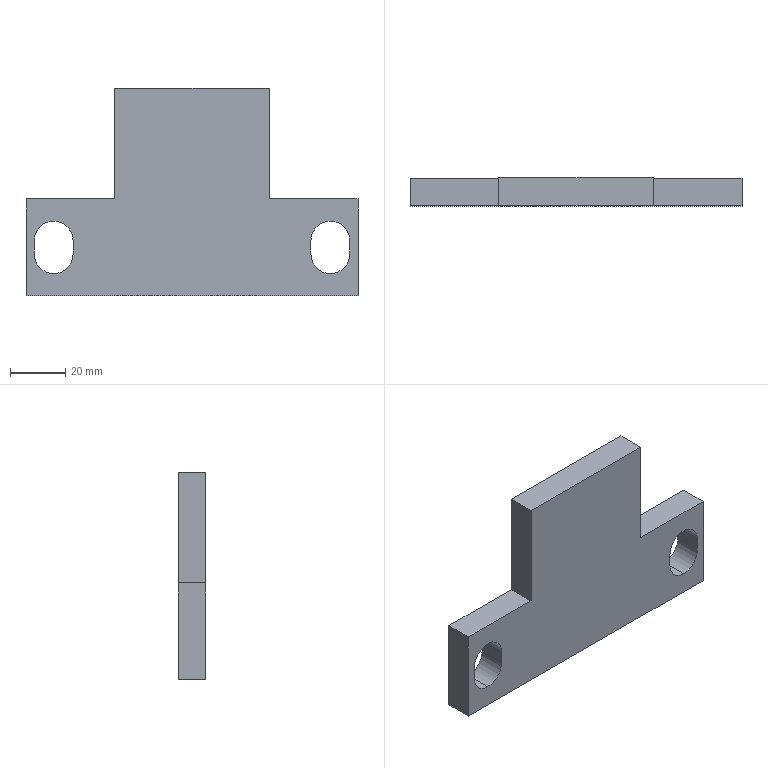Part | SolidWorks | features Extrusion 1 | 1 solid | 20 faces | box 120 x 10 x 75 mm | volume 59921 mm3 | plane 14 | cylinder 6 | commonest cylinder face diameters 14 x6
STEP:
#1=CARTESIAN_POINT('',(50.,10.,-29.5));
#2=VERTEX_POINT('',#1);
#3=CARTESIAN_POINT('',(57.,10.,-22.5));
#4=VERTEX_POINT('',#3);
#5=CARTESIAN_POINT('',(50.,10.,-22.5));
#6=DIRECTION('',(0.,-1.,0.));
#7=DIRECTION('',(0.,0.,1.));
#8=AXIS2_PLACEMENT_3D('',#5,#6,#7);
#9=CIRCLE('',#8,7.);
#10=EDGE_CURVE('',#2,#4,#9,.T.);
#11=ORIENTED_EDGE('',*,*,#10,.F.);
#12=CARTESIAN_POINT('',(50.,0.,-29.5));
#13=VERTEX_POINT('',#12);
#14=CARTESIAN_POINT('',(50.,10.,-29.5));
#15=DIRECTION('',(0.,-1.,0.));
#16=VECTOR('',#15,1000.);
#17=LINE('',#14,#16);
#18=EDGE_CURVE('',#2,#13,#17,.T.);
#19=ORIENTED_EDGE('',*,*,#18,.T.);
#20=CARTESIAN_POINT('',(57.,0.,-22.5));
#21=VERTEX_POINT('',#20);
#22=CARTESIAN_POINT('',(50.,0.,-22.5));
#23=DIRECTION('',(0.,-1.,0.));
#24=DIRECTION('',(0.,0.,1.));
#25=AXIS2_PLACEMENT_3D('',#22,#23,#24);
#26=CIRCLE('',#25,7.);
#27=EDGE_CURVE('',#13,#21,#26,.T.);
#28=ORIENTED_EDGE('',*,*,#27,.T.);
#29=CARTESIAN_POINT('',(57.,10.,-22.5));
#30=DIRECTION('',(0.,-1.,0.));
#31=VECTOR('',#30,1000.);
#32=LINE('',#29,#31);
#33=EDGE_CURVE('',#4,#21,#32,.T.);
#34=ORIENTED_EDGE('',*,*,#33,.F.);
#35=EDGE_LOOP('',(#11,#19,#28,#34));
#36=FACE_OUTER_BOUND('',#35,.T.);
#37=CARTESIAN_POINT('',(50.,10.,-22.5));
#38=DIRECTION('',(0.,-1.,0.));
#39=DIRECTION('',(0.,0.,-1.));
#40=AXIS2_PLACEMENT_3D('',#37,#38,#39);
#41=CYLINDRICAL_SURFACE('',#40,7.);
#42=ADVANCED_FACE('',(#36),#41,.F.);
#43=CARTESIAN_POINT('',(-43.,10.,-22.5));
#44=VERTEX_POINT('',#43);
#45=CARTESIAN_POINT('',(-50.,10.,-29.5));
#46=VERTEX_POINT('',#45);
#47=CARTESIAN_POINT('',(-50.,10.,-22.5));
#48=DIRECTION('',(0.,1.,0.));
#49=DIRECTION('',(0.,0.,1.));
#50=AXIS2_PLACEMENT_3D('',#47,#48,#49);
#51=CIRCLE('',#50,7.);
#52=EDGE_CURVE('',#44,#46,#51,.T.);
#53=ORIENTED_EDGE('',*,*,#52,.T.);
#54=CARTESIAN_POINT('',(-50.,0.,-29.5));
#55=VERTEX_POINT('',#54);
#56=CARTESIAN_POINT('',(-50.,10.,-29.5));
#57=DIRECTION('',(0.,-1.,0.));
#58=VECTOR('',#57,1000.);
#59=LINE('',#56,#58);
#60=EDGE_CURVE('',#46,#55,#59,.T.);
#61=ORIENTED_EDGE('',*,*,#60,.T.);
#62=CARTESIAN_POINT('',(-43.,0.,-22.5));
#63=VERTEX_POINT('',#62);
#64=CARTESIAN_POINT('',(-50.,0.,-22.5));
#65=DIRECTION('',(0.,1.,0.));
#66=DIRECTION('',(0.,0.,1.));
#67=AXIS2_PLACEMENT_3D('',#64,#65,#66);
#68=CIRCLE('',#67,7.);
#69=EDGE_CURVE('',#63,#55,#68,.T.);
#70=ORIENTED_EDGE('',*,*,#69,.F.);
#71=CARTESIAN_POINT('',(-43.,10.,-22.5));
#72=DIRECTION('',(0.,-1.,0.));
#73=VECTOR('',#72,1000.);
#74=LINE('',#71,#73);
#75=EDGE_CURVE('',#44,#63,#74,.T.);
#76=ORIENTED_EDGE('',*,*,#75,.F.);
#77=EDGE_LOOP('',(#53,#61,#70,#76));
#78=FACE_OUTER_BOUND('',#77,.T.);
#79=CARTESIAN_POINT('',(-50.,10.,-22.5));
#80=DIRECTION('',(0.,-1.,0.));
#81=DIRECTION('',(0.,0.,-1.));
#82=AXIS2_PLACEMENT_3D('',#79,#80,#81);
#83=CYLINDRICAL_SURFACE('',#82,7.);
#84=ADVANCED_FACE('',(#78),#83,.F.);
#85=CARTESIAN_POINT('',(57.,0.,-17.5));
#86=VERTEX_POINT('',#85);
#87=CARTESIAN_POINT('',(57.,0.,0.));
#88=DIRECTION('',(0.,0.,1.));
#89=VECTOR('',#88,1000.);
#90=LINE('',#87,#89);
#91=EDGE_CURVE('',#21,#86,#90,.T.);
#92=ORIENTED_EDGE('',*,*,#91,.T.);
#93=CARTESIAN_POINT('',(57.,10.,-17.5));
#94=VERTEX_POINT('',#93);
#95=CARTESIAN_POINT('',(57.,10.,-17.5));
#96=DIRECTION('',(0.,-1.,0.));
#97=VECTOR('',#96,1000.);
#98=LINE('',#95,#97);
#99=EDGE_CURVE('',#94,#86,#98,.T.);
#100=ORIENTED_EDGE('',*,*,#99,.F.);
#101=CARTESIAN_POINT('',(57.,10.,0.));
#102=DIRECTION('',(0.,0.,1.));
#103=VECTOR('',#102,1000.);
#104=LINE('',#101,#103);
#105=EDGE_CURVE('',#4,#94,#104,.T.);
#106=ORIENTED_EDGE('',*,*,#105,.F.);
#107=ORIENTED_EDGE('',*,*,#33,.T.);
#108=EDGE_LOOP('',(#92,#100,#106,#107));
#109=FACE_OUTER_BOUND('',#108,.T.);
#110=CARTESIAN_POINT('',(57.,10.,0.));
#111=DIRECTION('',(1.,0.,0.));
#112=DIRECTION('',(0.,0.,-1.));
#113=AXIS2_PLACEMENT_3D('',#110,#111,#112);
#114=PLANE('',#113);
#115=ADVANCED_FACE('',(#109),#114,.F.);
#116=CARTESIAN_POINT('',(43.,0.,-17.5));
#117=VERTEX_POINT('',#116);
#118=CARTESIAN_POINT('',(50.,0.,-17.5));
#119=DIRECTION('',(0.,-1.,0.));
#120=DIRECTION('',(0.,0.,1.));
#121=AXIS2_PLACEMENT_3D('',#118,#119,#120);
#122=CIRCLE('',#121,7.);
#123=EDGE_CURVE('',#86,#117,#122,.T.);
#124=ORIENTED_EDGE('',*,*,#123,.T.);
#125=CARTESIAN_POINT('',(43.,10.,-17.5));
#126=VERTEX_POINT('',#125);
#127=CARTESIAN_POINT('',(43.,10.,-17.5));
#128=DIRECTION('',(0.,-1.,0.));
#129=VECTOR('',#128,1000.);
#130=LINE('',#127,#129);
#131=EDGE_CURVE('',#126,#117,#130,.T.);
#132=ORIENTED_EDGE('',*,*,#131,.F.);
#133=CARTESIAN_POINT('',(50.,10.,-17.5));
#134=DIRECTION('',(0.,-1.,0.));
#135=DIRECTION('',(0.,0.,1.));
#136=AXIS2_PLACEMENT_3D('',#133,#134,#135);
#137=CIRCLE('',#136,7.);
#138=EDGE_CURVE('',#94,#126,#137,.T.);
#139=ORIENTED_EDGE('',*,*,#138,.F.);
#140=ORIENTED_EDGE('',*,*,#99,.T.);
#141=EDGE_LOOP('',(#124,#132,#139,#140));
#142=FACE_OUTER_BOUND('',#141,.T.);
#143=CARTESIAN_POINT('',(50.,10.,-17.5));
#144=DIRECTION('',(0.,-1.,0.));
#145=DIRECTION('',(0.,0.,-1.));
#146=AXIS2_PLACEMENT_3D('',#143,#144,#145);
#147=CYLINDRICAL_SURFACE('',#146,7.);
#148=ADVANCED_FACE('',(#142),#147,.F.);
#149=CARTESIAN_POINT('',(43.,0.,-22.5));
#150=VERTEX_POINT('',#149);
#151=CARTESIAN_POINT('',(43.,0.,0.));
#152=DIRECTION('',(0.,0.,1.));
#153=VECTOR('',#152,1000.);
#154=LINE('',#151,#153);
#155=EDGE_CURVE('',#150,#117,#154,.T.);
#156=ORIENTED_EDGE('',*,*,#155,.F.);
#157=CARTESIAN_POINT('',(43.,10.,-22.5));
#158=VERTEX_POINT('',#157);
#159=CARTESIAN_POINT('',(43.,10.,-22.5));
#160=DIRECTION('',(0.,-1.,0.));
#161=VECTOR('',#160,1000.);
#162=LINE('',#159,#161);
#163=EDGE_CURVE('',#158,#150,#162,.T.);
#164=ORIENTED_EDGE('',*,*,#163,.F.);
#165=CARTESIAN_POINT('',(43.,10.,0.));
#166=DIRECTION('',(0.,0.,1.));
#167=VECTOR('',#166,1000.);
#168=LINE('',#165,#167);
#169=EDGE_CURVE('',#158,#126,#168,.T.);
#170=ORIENTED_EDGE('',*,*,#169,.T.);
#171=ORIENTED_EDGE('',*,*,#131,.T.);
#172=EDGE_LOOP('',(#156,#164,#170,#171));
#173=FACE_OUTER_BOUND('',#172,.T.);
#174=CARTESIAN_POINT('',(43.,10.,0.));
#175=DIRECTION('',(1.,0.,0.));
#176=DIRECTION('',(0.,0.,-1.));
#177=AXIS2_PLACEMENT_3D('',#174,#175,#176);
#178=PLANE('',#177);
#179=ADVANCED_FACE('',(#173),#178,.T.);
#180=CARTESIAN_POINT('',(28.,0.,37.5));
#181=VERTEX_POINT('',#180);
#182=CARTESIAN_POINT('',(28.,0.,-2.5));
#183=VERTEX_POINT('',#182);
#184=CARTESIAN_POINT('',(28.,0.,0.));
#185=DIRECTION('',(0.,0.,-1.));
#186=VECTOR('',#185,1000.);
#187=LINE('',#184,#186);
#188=EDGE_CURVE('',#181,#183,#187,.T.);
#189=ORIENTED_EDGE('',*,*,#188,.T.);
#190=CARTESIAN_POINT('',(28.,10.,-2.5));
#191=VERTEX_POINT('',#190);
#192=CARTESIAN_POINT('',(28.,10.,-2.5));
#193=DIRECTION('',(0.,-1.,0.));
#194=VECTOR('',#193,1000.);
#195=LINE('',#192,#194);
#196=EDGE_CURVE('',#191,#183,#195,.T.);
#197=ORIENTED_EDGE('',*,*,#196,.F.);
#198=CARTESIAN_POINT('',(28.,10.,37.5));
#199=VERTEX_POINT('',#198);
#200=CARTESIAN_POINT('',(28.,10.,0.));
#201=DIRECTION('',(0.,0.,-1.));
#202=VECTOR('',#201,1000.);
#203=LINE('',#200,#202);
#204=EDGE_CURVE('',#199,#191,#203,.T.);
#205=ORIENTED_EDGE('',*,*,#204,.F.);
#206=CARTESIAN_POINT('',(28.,10.,37.5));
#207=DIRECTION('',(0.,-1.,0.));
#208=VECTOR('',#207,1000.);
#209=LINE('',#206,#208);
#210=EDGE_CURVE('',#199,#181,#209,.T.);
#211=ORIENTED_EDGE('',*,*,#210,.T.);
#212=EDGE_LOOP('',(#189,#197,#205,#211));
#213=FACE_OUTER_BOUND('',#212,.T.);
#214=CARTESIAN_POINT('',(28.,10.,0.));
#215=DIRECTION('',(-1.,0.,0.));
#216=DIRECTION('',(0.,0.,1.));
#217=AXIS2_PLACEMENT_3D('',#214,#215,#216);
#218=PLANE('',#217);
#219=ADVANCED_FACE('',(#213),#218,.F.);
#220=CARTESIAN_POINT('',(60.,0.,-2.5));
#221=VERTEX_POINT('',#220);
#222=CARTESIAN_POINT('',(0.,0.,-2.5));
#223=DIRECTION('',(1.,0.,0.));
#224=VECTOR('',#223,1000.);
#225=LINE('',#222,#224);
#226=EDGE_CURVE('',#183,#221,#225,.T.);
#227=ORIENTED_EDGE('',*,*,#226,.T.);
#228=CARTESIAN_POINT('',(60.,10.,-2.5));
#229=VERTEX_POINT('',#228);
#230=CARTESIAN_POINT('',(60.,10.,-2.5));
#231=DIRECTION('',(0.,-1.,0.));
#232=VECTOR('',#231,1000.);
#233=LINE('',#230,#232);
#234=EDGE_CURVE('',#229,#221,#233,.T.);
#235=ORIENTED_EDGE('',*,*,#234,.F.);
#236=CARTESIAN_POINT('',(0.,10.,-2.5));
#237=DIRECTION('',(1.,0.,0.));
#238=VECTOR('',#237,1000.);
#239=LINE('',#236,#238);
#240=EDGE_CURVE('',#191,#229,#239,.T.);
#241=ORIENTED_EDGE('',*,*,#240,.F.);
#242=ORIENTED_EDGE('',*,*,#196,.T.);
#243=EDGE_LOOP('',(#227,#235,#241,#242));
#244=FACE_OUTER_BOUND('',#243,.T.);
#245=CARTESIAN_POINT('',(0.,10.,-2.5));
#246=DIRECTION('',(0.,0.,-1.));
#247=DIRECTION('',(-1.,0.,0.));
#248=AXIS2_PLACEMENT_3D('',#245,#246,#247);
#249=PLANE('',#248);
#250=ADVANCED_FACE('',(#244),#249,.F.);
#251=CARTESIAN_POINT('',(60.,0.,-37.5));
#252=VERTEX_POINT('',#251);
#253=CARTESIAN_POINT('',(60.,0.,0.));
#254=DIRECTION('',(0.,0.,-1.));
#255=VECTOR('',#254,1000.);
#256=LINE('',#253,#255);
#257=EDGE_CURVE('',#221,#252,#256,.T.);
#258=ORIENTED_EDGE('',*,*,#257,.T.);
#259=CARTESIAN_POINT('',(60.,10.,-37.5));
#260=VERTEX_POINT('',#259);
#261=CARTESIAN_POINT('',(60.,10.,-37.5));
#262=DIRECTION('',(0.,-1.,0.));
#263=VECTOR('',#262,1000.);
#264=LINE('',#261,#263);
#265=EDGE_CURVE('',#260,#252,#264,.T.);
#266=ORIENTED_EDGE('',*,*,#265,.F.);
#267=CARTESIAN_POINT('',(60.,10.,0.));
#268=DIRECTION('',(0.,0.,-1.));
#269=VECTOR('',#268,1000.);
#270=LINE('',#267,#269);
#271=EDGE_CURVE('',#229,#260,#270,.T.);
#272=ORIENTED_EDGE('',*,*,#271,.F.);
#273=ORIENTED_EDGE('',*,*,#234,.T.);
#274=EDGE_LOOP('',(#258,#266,#272,#273));
#275=FACE_OUTER_BOUND('',#274,.T.);
#276=CARTESIAN_POINT('',(60.,10.,0.));
#277=DIRECTION('',(-1.,0.,0.));
#278=DIRECTION('',(0.,0.,1.));
#279=AXIS2_PLACEMENT_3D('',#276,#277,#278);
#280=PLANE('',#279);
#281=ADVANCED_FACE('',(#275),#280,.F.);
#282=CARTESIAN_POINT('',(-60.,0.,-37.5));
#283=VERTEX_POINT('',#282);
#284=CARTESIAN_POINT('',(0.,0.,-37.5));
#285=DIRECTION('',(1.,0.,0.));
#286=VECTOR('',#285,1000.);
#287=LINE('',#284,#286);
#288=EDGE_CURVE('',#283,#252,#287,.T.);
#289=ORIENTED_EDGE('',*,*,#288,.F.);
#290=CARTESIAN_POINT('',(-60.,10.,-37.5));
#291=VERTEX_POINT('',#290);
#292=CARTESIAN_POINT('',(-60.,10.,-37.5));
#293=DIRECTION('',(0.,-1.,0.));
#294=VECTOR('',#293,1000.);
#295=LINE('',#292,#294);
#296=EDGE_CURVE('',#291,#283,#295,.T.);
#297=ORIENTED_EDGE('',*,*,#296,.F.);
#298=CARTESIAN_POINT('',(0.,10.,-37.5));
#299=DIRECTION('',(1.,0.,0.));
#300=VECTOR('',#299,1000.);
#301=LINE('',#298,#300);
#302=EDGE_CURVE('',#291,#260,#301,.T.);
#303=ORIENTED_EDGE('',*,*,#302,.T.);
#304=ORIENTED_EDGE('',*,*,#265,.T.);
#305=EDGE_LOOP('',(#289,#297,#303,#304));
#306=FACE_OUTER_BOUND('',#305,.T.);
#307=CARTESIAN_POINT('',(0.,10.,-37.5));
#308=DIRECTION('',(0.,0.,-1.));
#309=DIRECTION('',(-1.,0.,0.));
#310=AXIS2_PLACEMENT_3D('',#307,#308,#309);
#311=PLANE('',#310);
#312=ADVANCED_FACE('',(#306),#311,.T.);
#313=CARTESIAN_POINT('',(-60.,0.,-2.5));
#314=VERTEX_POINT('',#313);
#315=CARTESIAN_POINT('',(-60.,0.,0.));
#316=DIRECTION('',(0.,0.,-1.));
#317=VECTOR('',#316,1000.);
#318=LINE('',#315,#317);
#319=EDGE_CURVE('',#314,#283,#318,.T.);
#320=ORIENTED_EDGE('',*,*,#319,.F.);
#321=CARTESIAN_POINT('',(-60.,10.,-2.5));
#322=VERTEX_POINT('',#321);
#323=CARTESIAN_POINT('',(-60.,10.,-2.5));
#324=DIRECTION('',(0.,-1.,0.));
#325=VECTOR('',#324,1000.);
#326=LINE('',#323,#325);
#327=EDGE_CURVE('',#322,#314,#326,.T.);
#328=ORIENTED_EDGE('',*,*,#327,.F.);
#329=CARTESIAN_POINT('',(-60.,10.,0.));
#330=DIRECTION('',(0.,0.,-1.));
#331=VECTOR('',#330,1000.);
#332=LINE('',#329,#331);
#333=EDGE_CURVE('',#322,#291,#332,.T.);
#334=ORIENTED_EDGE('',*,*,#333,.T.);
#335=ORIENTED_EDGE('',*,*,#296,.T.);
#336=EDGE_LOOP('',(#320,#328,#334,#335));
#337=FACE_OUTER_BOUND('',#336,.T.);
#338=CARTESIAN_POINT('',(-60.,10.,0.));
#339=DIRECTION('',(-1.,0.,0.));
#340=DIRECTION('',(0.,0.,1.));
#341=AXIS2_PLACEMENT_3D('',#338,#339,#340);
#342=PLANE('',#341);
#343=ADVANCED_FACE('',(#337),#342,.T.);
#344=CARTESIAN_POINT('',(-28.,0.,-2.5));
#345=VERTEX_POINT('',#344);
#346=CARTESIAN_POINT('',(0.,0.,-2.5));
#347=DIRECTION('',(1.,0.,0.));
#348=VECTOR('',#347,1000.);
#349=LINE('',#346,#348);
#350=EDGE_CURVE('',#314,#345,#349,.T.);
#351=ORIENTED_EDGE('',*,*,#350,.T.);
#352=CARTESIAN_POINT('',(-28.,10.,-2.5));
#353=VERTEX_POINT('',#352);
#354=CARTESIAN_POINT('',(-28.,10.,-2.5));
#355=DIRECTION('',(0.,-1.,0.));
#356=VECTOR('',#355,1000.);
#357=LINE('',#354,#356);
#358=EDGE_CURVE('',#353,#345,#357,.T.);
#359=ORIENTED_EDGE('',*,*,#358,.F.);
#360=CARTESIAN_POINT('',(0.,10.,-2.5));
#361=DIRECTION('',(1.,0.,0.));
#362=VECTOR('',#361,1000.);
#363=LINE('',#360,#362);
#364=EDGE_CURVE('',#322,#353,#363,.T.);
#365=ORIENTED_EDGE('',*,*,#364,.F.);
#366=ORIENTED_EDGE('',*,*,#327,.T.);
#367=EDGE_LOOP('',(#351,#359,#365,#366));
#368=FACE_OUTER_BOUND('',#367,.T.);
#369=CARTESIAN_POINT('',(0.,10.,-2.5));
#370=DIRECTION('',(0.,0.,-1.));
#371=DIRECTION('',(-1.,0.,0.));
#372=AXIS2_PLACEMENT_3D('',#369,#370,#371);
#373=PLANE('',#372);
#374=ADVANCED_FACE('',(#368),#373,.F.);
#375=CARTESIAN_POINT('',(-28.,0.,37.5));
#376=VERTEX_POINT('',#375);
#377=CARTESIAN_POINT('',(-28.,0.,0.));
#378=DIRECTION('',(0.,0.,1.));
#379=VECTOR('',#378,1000.);
#380=LINE('',#377,#379);
#381=EDGE_CURVE('',#345,#376,#380,.T.);
#382=ORIENTED_EDGE('',*,*,#381,.T.);
#383=CARTESIAN_POINT('',(-28.,10.,37.5));
#384=VERTEX_POINT('',#383);
#385=CARTESIAN_POINT('',(-28.,10.,37.5));
#386=DIRECTION('',(0.,-1.,0.));
#387=VECTOR('',#386,1000.);
#388=LINE('',#385,#387);
#389=EDGE_CURVE('',#384,#376,#388,.T.);
#390=ORIENTED_EDGE('',*,*,#389,.F.);
#391=CARTESIAN_POINT('',(-28.,10.,0.));
#392=DIRECTION('',(0.,0.,1.));
#393=VECTOR('',#392,1000.);
#394=LINE('',#391,#393);
#395=EDGE_CURVE('',#353,#384,#394,.T.);
#396=ORIENTED_EDGE('',*,*,#395,.F.);
#397=ORIENTED_EDGE('',*,*,#358,.T.);
#398=EDGE_LOOP('',(#382,#390,#396,#397));
#399=FACE_OUTER_BOUND('',#398,.T.);
#400=CARTESIAN_POINT('',(-28.,10.,0.));
#401=DIRECTION('',(1.,0.,0.));
#402=DIRECTION('',(0.,0.,-1.));
#403=AXIS2_PLACEMENT_3D('',#400,#401,#402);
#404=PLANE('',#403);
#405=ADVANCED_FACE('',(#399),#404,.F.);
#406=CARTESIAN_POINT('',(-57.,0.,-17.5));
#407=VERTEX_POINT('',#406);
#408=CARTESIAN_POINT('',(-43.,0.,-17.5));
#409=VERTEX_POINT('',#408);
#410=CARTESIAN_POINT('',(-50.,0.,-17.5));
#411=DIRECTION('',(0.,1.,0.));
#412=DIRECTION('',(0.,0.,1.));
#413=AXIS2_PLACEMENT_3D('',#410,#411,#412);
#414=CIRCLE('',#413,7.);
#415=EDGE_CURVE('',#407,#409,#414,.T.);
#416=ORIENTED_EDGE('',*,*,#415,.F.);
#417=CARTESIAN_POINT('',(-57.,10.,-17.5));
#418=VERTEX_POINT('',#417);
#419=CARTESIAN_POINT('',(-57.,10.,-17.5));
#420=DIRECTION('',(0.,-1.,0.));
#421=VECTOR('',#420,1000.);
#422=LINE('',#419,#421);
#423=EDGE_CURVE('',#418,#407,#422,.T.);
#424=ORIENTED_EDGE('',*,*,#423,.F.);
#425=CARTESIAN_POINT('',(-43.,10.,-17.5));
#426=VERTEX_POINT('',#425);
#427=CARTESIAN_POINT('',(-50.,10.,-17.5));
#428=DIRECTION('',(0.,1.,0.));
#429=DIRECTION('',(0.,0.,1.));
#430=AXIS2_PLACEMENT_3D('',#427,#428,#429);
#431=CIRCLE('',#430,7.);
#432=EDGE_CURVE('',#418,#426,#431,.T.);
#433=ORIENTED_EDGE('',*,*,#432,.T.);
#434=CARTESIAN_POINT('',(-43.,10.,-17.5));
#435=DIRECTION('',(0.,-1.,0.));
#436=VECTOR('',#435,1000.);
#437=LINE('',#434,#436);
#438=EDGE_CURVE('',#426,#409,#437,.T.);
#439=ORIENTED_EDGE('',*,*,#438,.T.);
#440=EDGE_LOOP('',(#416,#424,#433,#439));
#441=FACE_OUTER_BOUND('',#440,.T.);
#442=CARTESIAN_POINT('',(-50.,10.,-17.5));
#443=DIRECTION('',(0.,-1.,0.));
#444=DIRECTION('',(0.,0.,-1.));
#445=AXIS2_PLACEMENT_3D('',#442,#443,#444);
#446=CYLINDRICAL_SURFACE('',#445,7.);
#447=ADVANCED_FACE('',(#441),#446,.F.);
#448=CARTESIAN_POINT('',(-57.,0.,-22.5));
#449=VERTEX_POINT('',#448);
#450=CARTESIAN_POINT('',(-57.,0.,0.));
#451=DIRECTION('',(0.,0.,1.));
#452=VECTOR('',#451,1000.);
#453=LINE('',#450,#452);
#454=EDGE_CURVE('',#449,#407,#453,.T.);
#455=ORIENTED_EDGE('',*,*,#454,.F.);
#456=CARTESIAN_POINT('',(-57.,10.,-22.5));
#457=VERTEX_POINT('',#456);
#458=CARTESIAN_POINT('',(-57.,10.,-22.5));
#459=DIRECTION('',(0.,-1.,0.));
#460=VECTOR('',#459,1000.);
#461=LINE('',#458,#460);
#462=EDGE_CURVE('',#457,#449,#461,.T.);
#463=ORIENTED_EDGE('',*,*,#462,.F.);
#464=CARTESIAN_POINT('',(-57.,10.,0.));
#465=DIRECTION('',(0.,0.,1.));
#466=VECTOR('',#465,1000.);
#467=LINE('',#464,#466);
#468=EDGE_CURVE('',#457,#418,#467,.T.);
#469=ORIENTED_EDGE('',*,*,#468,.T.);
#470=ORIENTED_EDGE('',*,*,#423,.T.);
#471=EDGE_LOOP('',(#455,#463,#469,#470));
#472=FACE_OUTER_BOUND('',#471,.T.);
#473=CARTESIAN_POINT('',(-57.,10.,0.));
#474=DIRECTION('',(1.,0.,0.));
#475=DIRECTION('',(0.,0.,-1.));
#476=AXIS2_PLACEMENT_3D('',#473,#474,#475);
#477=PLANE('',#476);
#478=ADVANCED_FACE('',(#472),#477,.T.);
#479=ORIENTED_EDGE('',*,*,#60,.F.);
#480=CARTESIAN_POINT('',(-50.,10.,-22.5));
#481=DIRECTION('',(0.,1.,0.));
#482=DIRECTION('',(0.,0.,1.));
#483=AXIS2_PLACEMENT_3D('',#480,#481,#482);
#484=CIRCLE('',#483,7.);
#485=EDGE_CURVE('',#46,#457,#484,.T.);
#486=ORIENTED_EDGE('',*,*,#485,.T.);
#487=ORIENTED_EDGE('',*,*,#462,.T.);
#488=CARTESIAN_POINT('',(-50.,0.,-22.5));
#489=DIRECTION('',(0.,1.,0.));
#490=DIRECTION('',(0.,0.,1.));
#491=AXIS2_PLACEMENT_3D('',#488,#489,#490);
#492=CIRCLE('',#491,7.);
#493=EDGE_CURVE('',#55,#449,#492,.T.);
#494=ORIENTED_EDGE('',*,*,#493,.F.);
#495=EDGE_LOOP('',(#479,#486,#487,#494));
#496=FACE_OUTER_BOUND('',#495,.T.);
#497=CARTESIAN_POINT('',(-50.,10.,-22.5));
#498=DIRECTION('',(0.,-1.,0.));
#499=DIRECTION('',(0.,0.,-1.));
#500=AXIS2_PLACEMENT_3D('',#497,#498,#499);
#501=CYLINDRICAL_SURFACE('',#500,7.);
#502=ADVANCED_FACE('',(#496),#501,.F.);
#503=CARTESIAN_POINT('',(0.,0.,37.5));
#504=DIRECTION('',(1.,0.,0.));
#505=VECTOR('',#504,1000.);
#506=LINE('',#503,#505);
#507=EDGE_CURVE('',#376,#181,#506,.T.);
#508=ORIENTED_EDGE('',*,*,#507,.T.);
#509=ORIENTED_EDGE('',*,*,#210,.F.);
#510=CARTESIAN_POINT('',(0.,10.,37.5));
#511=DIRECTION('',(1.,0.,0.));
#512=VECTOR('',#511,1000.);
#513=LINE('',#510,#512);
#514=EDGE_CURVE('',#384,#199,#513,.T.);
#515=ORIENTED_EDGE('',*,*,#514,.F.);
#516=ORIENTED_EDGE('',*,*,#389,.T.);
#517=EDGE_LOOP('',(#508,#509,#515,#516));
#518=FACE_OUTER_BOUND('',#517,.T.);
#519=CARTESIAN_POINT('',(0.,10.,37.5));
#520=DIRECTION('',(0.,0.,-1.));
#521=DIRECTION('',(-1.,0.,0.));
#522=AXIS2_PLACEMENT_3D('',#519,#520,#521);
#523=PLANE('',#522);
#524=ADVANCED_FACE('',(#518),#523,.F.);
#525=CARTESIAN_POINT('',(-43.,0.,0.));
#526=DIRECTION('',(0.,0.,1.));
#527=VECTOR('',#526,1000.);
#528=LINE('',#525,#527);
#529=EDGE_CURVE('',#63,#409,#528,.T.);
#530=ORIENTED_EDGE('',*,*,#529,.T.);
#531=ORIENTED_EDGE('',*,*,#438,.F.);
#532=CARTESIAN_POINT('',(-43.,10.,0.));
#533=DIRECTION('',(0.,0.,1.));
#534=VECTOR('',#533,1000.);
#535=LINE('',#532,#534);
#536=EDGE_CURVE('',#44,#426,#535,.T.);
#537=ORIENTED_EDGE('',*,*,#536,.F.);
#538=ORIENTED_EDGE('',*,*,#75,.T.);
#539=EDGE_LOOP('',(#530,#531,#537,#538));
#540=FACE_OUTER_BOUND('',#539,.T.);
#541=CARTESIAN_POINT('',(-43.,10.,0.));
#542=DIRECTION('',(1.,0.,0.));
#543=DIRECTION('',(0.,0.,-1.));
#544=AXIS2_PLACEMENT_3D('',#541,#542,#543);
#545=PLANE('',#544);
#546=ADVANCED_FACE('',(#540),#545,.F.);
#547=ORIENTED_EDGE('',*,*,#18,.F.);
#548=CARTESIAN_POINT('',(50.,10.,-22.5));
#549=DIRECTION('',(0.,-1.,0.));
#550=DIRECTION('',(0.,0.,1.));
#551=AXIS2_PLACEMENT_3D('',#548,#549,#550);
#552=CIRCLE('',#551,7.);
#553=EDGE_CURVE('',#158,#2,#552,.T.);
#554=ORIENTED_EDGE('',*,*,#553,.F.);
#555=ORIENTED_EDGE('',*,*,#163,.T.);
#556=CARTESIAN_POINT('',(50.,0.,-22.5));
#557=DIRECTION('',(0.,-1.,0.));
#558=DIRECTION('',(0.,0.,1.));
#559=AXIS2_PLACEMENT_3D('',#556,#557,#558);
#560=CIRCLE('',#559,7.);
#561=EDGE_CURVE('',#150,#13,#560,.T.);
#562=ORIENTED_EDGE('',*,*,#561,.T.);
#563=EDGE_LOOP('',(#547,#554,#555,#562));
#564=FACE_OUTER_BOUND('',#563,.T.);
#565=CARTESIAN_POINT('',(50.,10.,-22.5));
#566=DIRECTION('',(0.,-1.,0.));
#567=DIRECTION('',(0.,0.,-1.));
#568=AXIS2_PLACEMENT_3D('',#565,#566,#567);
#569=CYLINDRICAL_SURFACE('',#568,7.);
#570=ADVANCED_FACE('',(#564),#569,.F.);
#571=ORIENTED_EDGE('',*,*,#432,.F.);
#572=ORIENTED_EDGE('',*,*,#468,.F.);
#573=ORIENTED_EDGE('',*,*,#485,.F.);
#574=ORIENTED_EDGE('',*,*,#52,.F.);
#575=ORIENTED_EDGE('',*,*,#536,.T.);
#576=EDGE_LOOP('',(#571,#572,#573,#574,#575));
#577=FACE_BOUND('',#576,.T.);
#578=ORIENTED_EDGE('',*,*,#204,.T.);
#579=ORIENTED_EDGE('',*,*,#240,.T.);
#580=ORIENTED_EDGE('',*,*,#271,.T.);
#581=ORIENTED_EDGE('',*,*,#302,.F.);
#582=ORIENTED_EDGE('',*,*,#333,.F.);
#583=ORIENTED_EDGE('',*,*,#364,.T.);
#584=ORIENTED_EDGE('',*,*,#395,.T.);
#585=ORIENTED_EDGE('',*,*,#514,.T.);
#586=EDGE_LOOP('',(#578,#579,#580,#581,#582,#583,#584,#585));
#587=FACE_OUTER_BOUND('',#586,.T.);
#588=ORIENTED_EDGE('',*,*,#105,.T.);
#589=ORIENTED_EDGE('',*,*,#138,.T.);
#590=ORIENTED_EDGE('',*,*,#169,.F.);
#591=ORIENTED_EDGE('',*,*,#553,.T.);
#592=ORIENTED_EDGE('',*,*,#10,.T.);
#593=EDGE_LOOP('',(#588,#589,#590,#591,#592));
#594=FACE_BOUND('',#593,.T.);
#595=CARTESIAN_POINT('',(0.,10.,0.));
#596=DIRECTION('',(0.,1.,0.));
#597=DIRECTION('',(0.,0.,1.));
#598=AXIS2_PLACEMENT_3D('',#595,#596,#597);
#599=PLANE('',#598);
#600=ADVANCED_FACE('',(#577,#587,#594),#599,.T.);
#601=ORIENTED_EDGE('',*,*,#415,.T.);
#602=ORIENTED_EDGE('',*,*,#529,.F.);
#603=ORIENTED_EDGE('',*,*,#69,.T.);
#604=ORIENTED_EDGE('',*,*,#493,.T.);
#605=ORIENTED_EDGE('',*,*,#454,.T.);
#606=EDGE_LOOP('',(#601,#602,#603,#604,#605));
#607=FACE_BOUND('',#606,.T.);
#608=ORIENTED_EDGE('',*,*,#188,.F.);
#609=ORIENTED_EDGE('',*,*,#507,.F.);
#610=ORIENTED_EDGE('',*,*,#381,.F.);
#611=ORIENTED_EDGE('',*,*,#350,.F.);
#612=ORIENTED_EDGE('',*,*,#319,.T.);
#613=ORIENTED_EDGE('',*,*,#288,.T.);
#614=ORIENTED_EDGE('',*,*,#257,.F.);
#615=ORIENTED_EDGE('',*,*,#226,.F.);
#616=EDGE_LOOP('',(#608,#609,#610,#611,#612,#613,#614,#615));
#617=FACE_OUTER_BOUND('',#616,.T.);
#618=ORIENTED_EDGE('',*,*,#91,.F.);
#619=ORIENTED_EDGE('',*,*,#27,.F.);
#620=ORIENTED_EDGE('',*,*,#561,.F.);
#621=ORIENTED_EDGE('',*,*,#155,.T.);
#622=ORIENTED_EDGE('',*,*,#123,.F.);
#623=EDGE_LOOP('',(#618,#619,#620,#621,#622));
#624=FACE_BOUND('',#623,.T.);
#625=CARTESIAN_POINT('',(0.,0.,0.));
#626=DIRECTION('',(0.,1.,0.));
#627=DIRECTION('',(0.,0.,1.));
#628=AXIS2_PLACEMENT_3D('',#625,#626,#627);
#629=PLANE('',#628);
#630=ADVANCED_FACE('',(#607,#617,#624),#629,.F.);
#631=CLOSED_SHELL('',(#42,#84,#115,#148,#179,#219,#250,#281,#312,#343,#374,#405,#447,#478,#502,#524,#546,#570,#600,#630));
#632=MANIFOLD_SOLID_BREP('',#631);
#633=CARTESIAN_POINT('',(0.,0.,0.));
#634=DIRECTION('',(0.,0.,1.));
#635=DIRECTION('',(1.,0.,0.));
#636=AXIS2_PLACEMENT_3D('',#633,#634,#635);
#637=(LENGTH_UNIT()NAMED_UNIT(*)SI_UNIT(.MILLI.,.METRE.));
#638=UNCERTAINTY_MEASURE_WITH_UNIT(LENGTH_MEASURE(0.00001),#637,'','');
#639=(NAMED_UNIT(*)PLANE_ANGLE_UNIT()SI_UNIT($,.RADIAN.));
#640=(NAMED_UNIT(*)SI_UNIT($,.STERADIAN.)SOLID_ANGLE_UNIT());
#641=(GEOMETRIC_REPRESENTATION_CONTEXT(3)GLOBAL_UNCERTAINTY_ASSIGNED_CONTEXT((#638))GLOBAL_UNIT_ASSIGNED_CONTEXT((#637,#639,#640))REPRESENTATION_CONTEXT('',''));
#642=ADVANCED_BREP_SHAPE_REPRESENTATION('',(#632,#636),#641);